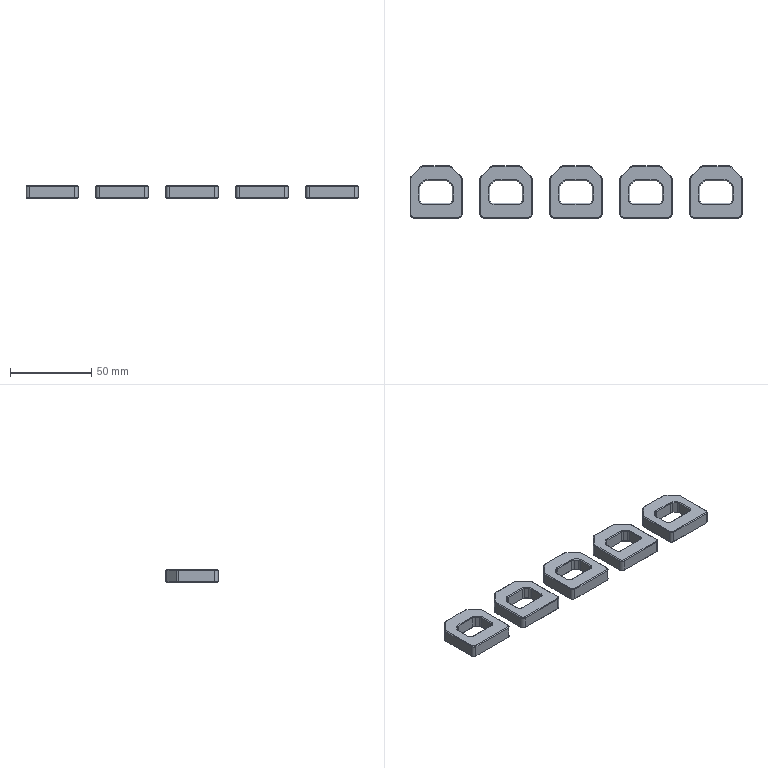Part | 5 solids | 470 faces | box 204 x 32 x 8 mm | volume 26393 mm3 | plane 210 | cone 160 | cylinder 100 | commonest cylinder face diameters 4 x100